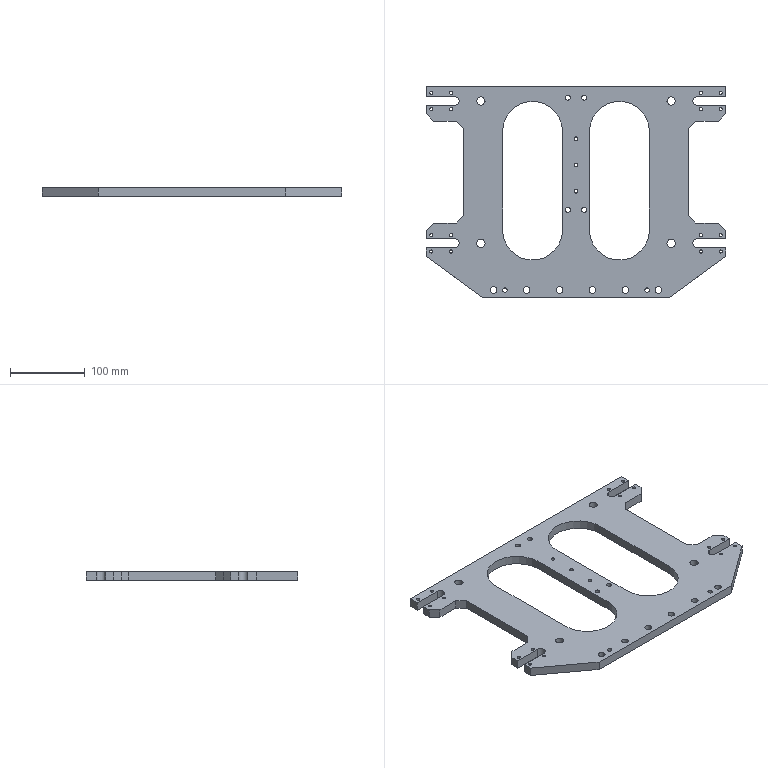Part | 1 solid | 83 faces | box 400 x 282 x 12 mm | volume 727391 mm3 | cylinder 43 | plane 40 | commonest cylinder face diameters 4.2 x16 9 x6 6.6 x4 11 x4 12 x4 80 x4